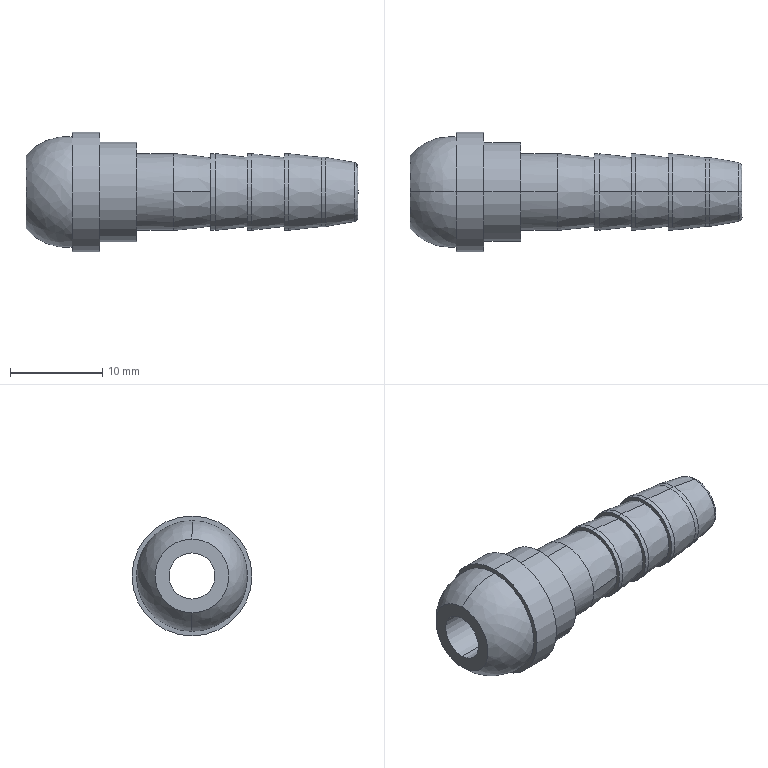Part | STEP file | 20C | 1 solid | 38 faces | box 36 x 13 x 13 mm | volume 1696 mm3 | cylinder 16 | cone 10 | plane 8 | spline 4 | commonest cylinder face diameters 8.3 x4 8.341 x4 5 x2 7.5 x2 10.8 x2 13 x2
STEP:
#1=CARTESIAN_POINT('',(44.153,0.,3.206));
#2=VERTEX_POINT('',#1);
#3=CARTESIAN_POINT('',(44.153,0.,-3.206));
#4=VERTEX_POINT('',#3);
#5=CARTESIAN_POINT('',(44.153,0.,0.));
#6=DIRECTION('',(1.,0.,0.));
#7=DIRECTION('',(0.,0.,1.));
#8=AXIS2_PLACEMENT_3D('',#5,#6,#7);
#9=CIRCLE('',#8,3.206);
#10=EDGE_CURVE('',#2,#4,#9,.T.);
#11=ORIENTED_EDGE('',*,*,#10,.T.);
#12=CARTESIAN_POINT('',(44.566,0.,-2.713));
#13=VERTEX_POINT('',#12);
#14=CARTESIAN_POINT('',(44.066,0.,-2.713));
#15=DIRECTION('',(0.,-1.,0.));
#16=DIRECTION('',(0.,0.,-1.));
#17=AXIS2_PLACEMENT_3D('',#14,#15,#16);
#18=CIRCLE('',#17,0.5);
#19=EDGE_CURVE('',#4,#13,#18,.T.);
#20=ORIENTED_EDGE('',*,*,#19,.T.);
#21=CARTESIAN_POINT('',(44.566,0.,2.713));
#22=VERTEX_POINT('',#21);
#23=CARTESIAN_POINT('',(44.566,0.,-2.713));
#24=CARTESIAN_POINT('',(44.566,-5.427,-2.713));
#25=CARTESIAN_POINT('',(44.566,-5.427,2.713));
#26=CARTESIAN_POINT('',(44.566,0.,2.713));
#27=(BOUNDED_CURVE()B_SPLINE_CURVE(3,(#23,#24,#25,#26),.UNSPECIFIED.,.F.,.F.)B_SPLINE_CURVE_WITH_KNOTS((4,4),(0.,1.),.UNSPECIFIED.)CURVE()GEOMETRIC_REPRESENTATION_ITEM()RATIONAL_B_SPLINE_CURVE((1.,0.3333,0.3333,1.))REPRESENTATION_ITEM(''));
#28=EDGE_CURVE('',#13,#22,#27,.T.);
#29=ORIENTED_EDGE('',*,*,#28,.T.);
#30=CARTESIAN_POINT('',(44.066,0.,2.713));
#31=DIRECTION('',(0.,1.,0.));
#32=DIRECTION('',(0.,0.,1.));
#33=AXIS2_PLACEMENT_3D('',#30,#31,#32);
#34=CIRCLE('',#33,0.5);
#35=EDGE_CURVE('',#2,#22,#34,.T.);
#36=ORIENTED_EDGE('',*,*,#35,.F.);
#37=EDGE_LOOP('',(#11,#20,#29,#36));
#38=FACE_OUTER_BOUND('',#37,.T.);
#39=CARTESIAN_POINT('',(44.153,0.,-3.206));
#40=CARTESIAN_POINT('',(44.153,-6.411,-3.206));
#41=CARTESIAN_POINT('',(44.153,-6.411,3.206));
#42=CARTESIAN_POINT('',(44.153,0.,3.206));
#43=CARTESIAN_POINT('',(44.403,0.,-3.162));
#44=CARTESIAN_POINT('',(44.403,-6.323,-3.162));
#45=CARTESIAN_POINT('',(44.403,-6.323,3.162));
#46=CARTESIAN_POINT('',(44.403,0.,3.162));
#47=CARTESIAN_POINT('',(44.566,0.,-2.967));
#48=CARTESIAN_POINT('',(44.566,-5.934,-2.967));
#49=CARTESIAN_POINT('',(44.566,-5.934,2.967));
#50=CARTESIAN_POINT('',(44.566,0.,2.967));
#51=CARTESIAN_POINT('',(44.566,0.,-2.713));
#52=CARTESIAN_POINT('',(44.566,-5.427,-2.713));
#53=CARTESIAN_POINT('',(44.566,-5.427,2.713));
#54=CARTESIAN_POINT('',(44.566,0.,2.713));
#55=(BOUNDED_SURFACE()B_SPLINE_SURFACE(3,3,((#39,#40,#41,#42),(#43,#44,#45,#46),(#47,#48,#49,#50),(#51,#52,#53,#54)),.UNSPECIFIED.,.F.,.F.,.F.)B_SPLINE_SURFACE_WITH_KNOTS((4,4),(4,4),(0.,1.),(0.,1.),.UNSPECIFIED.)GEOMETRIC_REPRESENTATION_ITEM()RATIONAL_B_SPLINE_SURFACE(((1.,0.3333,0.3333,1.),(0.844,0.2813,0.2813,0.844),(0.844,0.2813,0.2813,0.844),(1.,0.3333,0.3333,1.)))REPRESENTATION_ITEM('')SURFACE());
#56=ADVANCED_FACE('',(#38),#55,.T.);
#57=CARTESIAN_POINT('',(8.566,0.,4.));
#58=VERTEX_POINT('',#57);
#59=CARTESIAN_POINT('',(8.566,0.,-4.));
#60=VERTEX_POINT('',#59);
#61=CARTESIAN_POINT('',(8.566,0.,0.));
#62=DIRECTION('',(1.,0.,0.));
#63=DIRECTION('',(0.,0.,1.));
#64=AXIS2_PLACEMENT_3D('',#61,#62,#63);
#65=CIRCLE('',#64,4.);
#66=EDGE_CURVE('',#58,#60,#65,.T.);
#67=ORIENTED_EDGE('',*,*,#66,.T.);
#68=CARTESIAN_POINT('',(13.566,0.,-6.));
#69=VERTEX_POINT('',#68);
#70=CARTESIAN_POINT('',(13.057,0.,-0.0216));
#71=DIRECTION('',(0.,-1.,0.));
#72=DIRECTION('',(0.,0.,-1.));
#73=AXIS2_PLACEMENT_3D('',#70,#71,#72);
#74=CIRCLE('',#73,6.);
#75=EDGE_CURVE('',#60,#69,#74,.T.);
#76=ORIENTED_EDGE('',*,*,#75,.T.);
#77=CARTESIAN_POINT('',(13.566,0.,6.));
#78=VERTEX_POINT('',#77);
#79=CARTESIAN_POINT('',(13.566,0.,0.));
#80=DIRECTION('',(-1.,0.,0.));
#81=DIRECTION('',(0.,0.,1.));
#82=AXIS2_PLACEMENT_3D('',#79,#80,#81);
#83=CIRCLE('',#82,6.);
#84=EDGE_CURVE('',#69,#78,#83,.T.);
#85=ORIENTED_EDGE('',*,*,#84,.T.);
#86=CARTESIAN_POINT('',(13.057,0.,0.0216));
#87=DIRECTION('',(0.,1.,0.));
#88=DIRECTION('',(0.,0.,1.));
#89=AXIS2_PLACEMENT_3D('',#86,#87,#88);
#90=CIRCLE('',#89,6.);
#91=EDGE_CURVE('',#58,#78,#90,.T.);
#92=ORIENTED_EDGE('',*,*,#91,.F.);
#93=EDGE_LOOP('',(#67,#76,#85,#92));
#94=FACE_OUTER_BOUND('',#93,.T.);
#95=CARTESIAN_POINT('',(8.566,0.,-4.));
#96=CARTESIAN_POINT('',(8.566,-8.,-4.));
#97=CARTESIAN_POINT('',(8.566,-8.,4.));
#98=CARTESIAN_POINT('',(8.566,0.,4.));
#99=CARTESIAN_POINT('',(9.847,0.,-5.446));
#100=CARTESIAN_POINT('',(9.847,-10.892,-5.446));
#101=CARTESIAN_POINT('',(9.847,-10.892,5.446));
#102=CARTESIAN_POINT('',(9.847,0.,5.446));
#103=CARTESIAN_POINT('',(11.641,0.,-6.164));
#104=CARTESIAN_POINT('',(11.641,-12.328,-6.164));
#105=CARTESIAN_POINT('',(11.641,-12.328,6.164));
#106=CARTESIAN_POINT('',(11.641,0.,6.164));
#107=CARTESIAN_POINT('',(13.566,0.,-6.));
#108=CARTESIAN_POINT('',(13.566,-12.,-6.));
#109=CARTESIAN_POINT('',(13.566,-12.,6.));
#110=CARTESIAN_POINT('',(13.566,0.,6.));
#111=(BOUNDED_SURFACE()B_SPLINE_SURFACE(3,3,((#95,#96,#97,#98),(#99,#100,#101,#102),(#103,#104,#105,#106),(#107,#108,#109,#110)),.UNSPECIFIED.,.F.,.F.,.T.)B_SPLINE_SURFACE_WITH_KNOTS((4,4),(4,4),(0.,1.),(0.,1.),.UNSPECIFIED.)GEOMETRIC_REPRESENTATION_ITEM()RATIONAL_B_SPLINE_SURFACE(((1.,0.3333,0.3333,1.),(0.9291,0.3097,0.3097,0.9291),(0.9291,0.3097,0.3097,0.9291),(1.,0.3333,0.3333,1.)))REPRESENTATION_ITEM('')SURFACE());
#112=ADVANCED_FACE('',(#94),#111,.T.);
#113=CARTESIAN_POINT('',(44.566,0.,-2.5));
#114=VERTEX_POINT('',#113);
#115=CARTESIAN_POINT('',(44.566,0.,2.5));
#116=VERTEX_POINT('',#115);
#117=CARTESIAN_POINT('',(44.566,0.,0.));
#118=DIRECTION('',(-1.,0.,0.));
#119=DIRECTION('',(0.,0.,1.));
#120=AXIS2_PLACEMENT_3D('',#117,#118,#119);
#121=CIRCLE('',#120,2.5);
#122=EDGE_CURVE('',#114,#116,#121,.T.);
#123=ORIENTED_EDGE('',*,*,#122,.F.);
#124=CARTESIAN_POINT('',(8.566,0.,-2.5));
#125=VERTEX_POINT('',#124);
#126=CARTESIAN_POINT('',(-40.973,0.,-2.5));
#127=DIRECTION('',(-1.,0.,0.));
#128=VECTOR('',#127,1000.);
#129=LINE('',#126,#128);
#130=EDGE_CURVE('',#114,#125,#129,.T.);
#131=ORIENTED_EDGE('',*,*,#130,.T.);
#132=CARTESIAN_POINT('',(8.566,0.,2.5));
#133=VERTEX_POINT('',#132);
#134=CARTESIAN_POINT('',(8.566,0.,0.));
#135=DIRECTION('',(1.,0.,0.));
#136=DIRECTION('',(0.,0.,1.));
#137=AXIS2_PLACEMENT_3D('',#134,#135,#136);
#138=CIRCLE('',#137,2.5);
#139=EDGE_CURVE('',#133,#125,#138,.T.);
#140=ORIENTED_EDGE('',*,*,#139,.F.);
#141=CARTESIAN_POINT('',(-40.973,0.,2.5));
#142=DIRECTION('',(-1.,0.,0.));
#143=VECTOR('',#142,1000.);
#144=LINE('',#141,#143);
#145=EDGE_CURVE('',#116,#133,#144,.T.);
#146=ORIENTED_EDGE('',*,*,#145,.F.);
#147=EDGE_LOOP('',(#123,#131,#140,#146));
#148=FACE_OUTER_BOUND('',#147,.T.);
#149=CARTESIAN_POINT('',(-40.973,0.,0.));
#150=DIRECTION('',(-1.,0.,0.));
#151=DIRECTION('',(0.,0.,1.));
#152=AXIS2_PLACEMENT_3D('',#149,#150,#151);
#153=CYLINDRICAL_SURFACE('',#152,2.5);
#154=ADVANCED_FACE('',(#148),#153,.F.);
#155=CARTESIAN_POINT('',(44.153,0.,0.));
#156=DIRECTION('',(1.,0.,0.));
#157=DIRECTION('',(0.,0.,1.));
#158=AXIS2_PLACEMENT_3D('',#155,#156,#157);
#159=CIRCLE('',#158,3.206);
#160=EDGE_CURVE('',#4,#2,#159,.T.);
#161=ORIENTED_EDGE('',*,*,#160,.F.);
#162=CARTESIAN_POINT('',(41.066,0.,-3.75));
#163=VERTEX_POINT('',#162);
#164=CARTESIAN_POINT('',(41.066,0.,-3.75));
#165=DIRECTION('',(-0.9848,0.,-0.1736));
#166=VECTOR('',#165,1000.);
#167=LINE('',#164,#166);
#168=EDGE_CURVE('',#4,#163,#167,.T.);
#169=ORIENTED_EDGE('',*,*,#168,.T.);
#170=CARTESIAN_POINT('',(41.066,0.,3.75));
#171=VERTEX_POINT('',#170);
#172=CARTESIAN_POINT('',(41.066,0.,0.));
#173=DIRECTION('',(1.,0.,0.));
#174=DIRECTION('',(0.,0.,1.));
#175=AXIS2_PLACEMENT_3D('',#172,#173,#174);
#176=CIRCLE('',#175,3.75);
#177=EDGE_CURVE('',#163,#171,#176,.T.);
#178=ORIENTED_EDGE('',*,*,#177,.T.);
#179=CARTESIAN_POINT('',(41.066,0.,3.75));
#180=DIRECTION('',(-0.9848,0.,0.1736));
#181=VECTOR('',#180,1000.);
#182=LINE('',#179,#181);
#183=EDGE_CURVE('',#2,#171,#182,.T.);
#184=ORIENTED_EDGE('',*,*,#183,.F.);
#185=EDGE_LOOP('',(#161,#169,#178,#184));
#186=FACE_OUTER_BOUND('',#185,.T.);
#187=CARTESIAN_POINT('',(41.066,0.,0.));
#188=DIRECTION('',(-1.,0.,0.));
#189=DIRECTION('',(0.,0.,1.));
#190=AXIS2_PLACEMENT_3D('',#187,#188,#189);
#191=CONICAL_SURFACE('',#190,3.75,0.1745);
#192=ADVANCED_FACE('',(#186),#191,.T.);
#193=ORIENTED_EDGE('',*,*,#177,.F.);
#194=CARTESIAN_POINT('',(40.566,0.,-3.75));
#195=VERTEX_POINT('',#194);
#196=CARTESIAN_POINT('',(-40.973,0.,-3.75));
#197=DIRECTION('',(-1.,0.,0.));
#198=VECTOR('',#197,1000.);
#199=LINE('',#196,#198);
#200=EDGE_CURVE('',#163,#195,#199,.T.);
#201=ORIENTED_EDGE('',*,*,#200,.T.);
#202=CARTESIAN_POINT('',(40.566,0.,3.75));
#203=VERTEX_POINT('',#202);
#204=CARTESIAN_POINT('',(40.566,0.,0.));
#205=DIRECTION('',(1.,0.,0.));
#206=DIRECTION('',(0.,0.,1.));
#207=AXIS2_PLACEMENT_3D('',#204,#205,#206);
#208=CIRCLE('',#207,3.75);
#209=EDGE_CURVE('',#195,#203,#208,.T.);
#210=ORIENTED_EDGE('',*,*,#209,.T.);
#211=CARTESIAN_POINT('',(-40.973,0.,3.75));
#212=DIRECTION('',(-1.,0.,0.));
#213=VECTOR('',#212,1000.);
#214=LINE('',#211,#213);
#215=EDGE_CURVE('',#171,#203,#214,.T.);
#216=ORIENTED_EDGE('',*,*,#215,.F.);
#217=EDGE_LOOP('',(#193,#201,#210,#216));
#218=FACE_OUTER_BOUND('',#217,.T.);
#219=CARTESIAN_POINT('',(-40.973,0.,0.));
#220=DIRECTION('',(-1.,0.,0.));
#221=DIRECTION('',(0.,0.,1.));
#222=AXIS2_PLACEMENT_3D('',#219,#220,#221);
#223=CYLINDRICAL_SURFACE('',#222,3.75);
#224=ADVANCED_FACE('',(#218),#223,.T.);
#225=CARTESIAN_POINT('',(16.566,0.,6.5));
#226=VERTEX_POINT('',#225);
#227=CARTESIAN_POINT('',(16.566,0.,-6.5));
#228=VERTEX_POINT('',#227);
#229=CARTESIAN_POINT('',(16.566,0.,0.));
#230=DIRECTION('',(-1.,0.,0.));
#231=DIRECTION('',(0.,0.,1.));
#232=AXIS2_PLACEMENT_3D('',#229,#230,#231);
#233=CIRCLE('',#232,6.5);
#234=EDGE_CURVE('',#226,#228,#233,.T.);
#235=ORIENTED_EDGE('',*,*,#234,.T.);
#236=CARTESIAN_POINT('',(13.566,0.,-6.5));
#237=VERTEX_POINT('',#236);
#238=CARTESIAN_POINT('',(-40.973,0.,-6.5));
#239=DIRECTION('',(-1.,0.,0.));
#240=VECTOR('',#239,1000.);
#241=LINE('',#238,#240);
#242=EDGE_CURVE('',#228,#237,#241,.T.);
#243=ORIENTED_EDGE('',*,*,#242,.T.);
#244=CARTESIAN_POINT('',(13.566,0.,6.5));
#245=VERTEX_POINT('',#244);
#246=CARTESIAN_POINT('',(13.566,0.,0.));
#247=DIRECTION('',(1.,0.,0.));
#248=DIRECTION('',(0.,0.,1.));
#249=AXIS2_PLACEMENT_3D('',#246,#247,#248);
#250=CIRCLE('',#249,6.5);
#251=EDGE_CURVE('',#237,#245,#250,.T.);
#252=ORIENTED_EDGE('',*,*,#251,.T.);
#253=CARTESIAN_POINT('',(-40.973,0.,6.5));
#254=DIRECTION('',(-1.,0.,0.));
#255=VECTOR('',#254,1000.);
#256=LINE('',#253,#255);
#257=EDGE_CURVE('',#226,#245,#256,.T.);
#258=ORIENTED_EDGE('',*,*,#257,.F.);
#259=EDGE_LOOP('',(#235,#243,#252,#258));
#260=FACE_OUTER_BOUND('',#259,.T.);
#261=CARTESIAN_POINT('',(-40.973,0.,0.));
#262=DIRECTION('',(-1.,0.,0.));
#263=DIRECTION('',(0.,0.,1.));
#264=AXIS2_PLACEMENT_3D('',#261,#262,#263);
#265=CYLINDRICAL_SURFACE('',#264,6.5);
#266=ADVANCED_FACE('',(#260),#265,.T.);
#267=ORIENTED_EDGE('',*,*,#209,.F.);
#268=CARTESIAN_POINT('',(37.066,0.,-4.15));
#269=VERTEX_POINT('',#268);
#270=CARTESIAN_POINT('',(37.066,0.,-4.15));
#271=DIRECTION('',(-0.9935,0.,-0.1135));
#272=VECTOR('',#271,1000.);
#273=LINE('',#270,#272);
#274=EDGE_CURVE('',#195,#269,#273,.T.);
#275=ORIENTED_EDGE('',*,*,#274,.T.);
#276=CARTESIAN_POINT('',(37.066,0.,4.15));
#277=VERTEX_POINT('',#276);
#278=CARTESIAN_POINT('',(37.066,0.,0.));
#279=DIRECTION('',(1.,0.,0.));
#280=DIRECTION('',(0.,0.,1.));
#281=AXIS2_PLACEMENT_3D('',#278,#279,#280);
#282=CIRCLE('',#281,4.15);
#283=EDGE_CURVE('',#269,#277,#282,.T.);
#284=ORIENTED_EDGE('',*,*,#283,.T.);
#285=CARTESIAN_POINT('',(37.066,0.,4.15));
#286=DIRECTION('',(-0.9935,0.,0.1135));
#287=VECTOR('',#286,1000.);
#288=LINE('',#285,#287);
#289=EDGE_CURVE('',#203,#277,#288,.T.);
#290=ORIENTED_EDGE('',*,*,#289,.F.);
#291=EDGE_LOOP('',(#267,#275,#284,#290));
#292=FACE_OUTER_BOUND('',#291,.T.);
#293=CARTESIAN_POINT('',(37.066,0.,0.));
#294=DIRECTION('',(-1.,0.,0.));
#295=DIRECTION('',(0.,0.,1.));
#296=AXIS2_PLACEMENT_3D('',#293,#294,#295);
#297=CONICAL_SURFACE('',#296,4.15,0.1138);
#298=ADVANCED_FACE('',(#292),#297,.T.);
#299=ORIENTED_EDGE('',*,*,#283,.F.);
#300=CARTESIAN_POINT('',(36.566,0.,-4.15));
#301=VERTEX_POINT('',#300);
#302=CARTESIAN_POINT('',(-40.973,0.,-4.15));
#303=DIRECTION('',(-1.,0.,0.));
#304=VECTOR('',#303,1000.);
#305=LINE('',#302,#304);
#306=EDGE_CURVE('',#269,#301,#305,.T.);
#307=ORIENTED_EDGE('',*,*,#306,.T.);
#308=CARTESIAN_POINT('',(36.566,0.,4.15));
#309=VERTEX_POINT('',#308);
#310=CARTESIAN_POINT('',(36.566,0.,0.));
#311=DIRECTION('',(1.,0.,0.));
#312=DIRECTION('',(0.,0.,1.));
#313=AXIS2_PLACEMENT_3D('',#310,#311,#312);
#314=CIRCLE('',#313,4.15);
#315=EDGE_CURVE('',#301,#309,#314,.T.);
#316=ORIENTED_EDGE('',*,*,#315,.T.);
#317=CARTESIAN_POINT('',(-40.973,0.,4.15));
#318=DIRECTION('',(-1.,0.,0.));
#319=VECTOR('',#318,1000.);
#320=LINE('',#317,#319);
#321=EDGE_CURVE('',#277,#309,#320,.T.);
#322=ORIENTED_EDGE('',*,*,#321,.F.);
#323=EDGE_LOOP('',(#299,#307,#316,#322));
#324=FACE_OUTER_BOUND('',#323,.T.);
#325=CARTESIAN_POINT('',(-40.973,0.,0.));
#326=DIRECTION('',(-1.,0.,0.));
#327=DIRECTION('',(0.,0.,1.));
#328=AXIS2_PLACEMENT_3D('',#325,#326,#327);
#329=CYLINDRICAL_SURFACE('',#328,4.15);
#330=ADVANCED_FACE('',(#324),#329,.T.);
#331=CARTESIAN_POINT('',(20.566,0.,5.4));
#332=VERTEX_POINT('',#331);
#333=CARTESIAN_POINT('',(20.566,0.,-5.4));
#334=VERTEX_POINT('',#333);
#335=CARTESIAN_POINT('',(20.566,0.,0.));
#336=DIRECTION('',(-1.,0.,0.));
#337=DIRECTION('',(0.,0.,1.));
#338=AXIS2_PLACEMENT_3D('',#335,#336,#337);
#339=CIRCLE('',#338,5.4);
#340=EDGE_CURVE('',#332,#334,#339,.T.);
#341=ORIENTED_EDGE('',*,*,#340,.T.);
#342=CARTESIAN_POINT('',(16.566,0.,-5.4));
#343=VERTEX_POINT('',#342);
#344=CARTESIAN_POINT('',(-40.973,0.,-5.4));
#345=DIRECTION('',(-1.,0.,0.));
#346=VECTOR('',#345,1000.);
#347=LINE('',#344,#346);
#348=EDGE_CURVE('',#334,#343,#347,.T.);
#349=ORIENTED_EDGE('',*,*,#348,.T.);
#350=CARTESIAN_POINT('',(16.566,0.,5.4));
#351=VERTEX_POINT('',#350);
#352=CARTESIAN_POINT('',(16.566,0.,0.));
#353=DIRECTION('',(1.,0.,0.));
#354=DIRECTION('',(0.,0.,1.));
#355=AXIS2_PLACEMENT_3D('',#352,#353,#354);
#356=CIRCLE('',#355,5.4);
#357=EDGE_CURVE('',#343,#351,#356,.T.);
#358=ORIENTED_EDGE('',*,*,#357,.T.);
#359=CARTESIAN_POINT('',(-40.973,0.,5.4));
#360=DIRECTION('',(-1.,0.,0.));
#361=VECTOR('',#360,1000.);
#362=LINE('',#359,#361);
#363=EDGE_CURVE('',#332,#351,#362,.T.);
#364=ORIENTED_EDGE('',*,*,#363,.F.);
#365=EDGE_LOOP('',(#341,#349,#358,#364));
#366=FACE_OUTER_BOUND('',#365,.T.);
#367=CARTESIAN_POINT('',(-40.973,0.,0.));
#368=DIRECTION('',(-1.,0.,0.));
#369=DIRECTION('',(0.,0.,1.));
#370=AXIS2_PLACEMENT_3D('',#367,#368,#369);
#371=CYLINDRICAL_SURFACE('',#370,5.4);
#372=ADVANCED_FACE('',(#366),#371,.T.);
#373=CARTESIAN_POINT('',(36.566,0.,3.73));
#374=VERTEX_POINT('',#373);
#375=CARTESIAN_POINT('',(36.566,0.,-3.73));
#376=VERTEX_POINT('',#375);
#377=CARTESIAN_POINT('',(36.566,0.,0.));
#378=DIRECTION('',(-1.,0.,0.));
#379=DIRECTION('',(0.,0.,1.));
#380=AXIS2_PLACEMENT_3D('',#377,#378,#379);
#381=CIRCLE('',#380,3.73);
#382=EDGE_CURVE('',#374,#376,#381,.T.);
#383=ORIENTED_EDGE('',*,*,#382,.T.);
#384=CARTESIAN_POINT('',(33.066,0.,-4.15));
#385=VERTEX_POINT('',#384);
#386=CARTESIAN_POINT('',(33.066,0.,-4.15));
#387=DIRECTION('',(-0.9929,0.,-0.1192));
#388=VECTOR('',#387,1000.);
#389=LINE('',#386,#388);
#390=EDGE_CURVE('',#376,#385,#389,.T.);
#391=ORIENTED_EDGE('',*,*,#390,.T.);
#392=CARTESIAN_POINT('',(33.066,0.,4.15));
#393=VERTEX_POINT('',#392);
#394=CARTESIAN_POINT('',(33.066,0.,0.));
#395=DIRECTION('',(1.,0.,0.));
#396=DIRECTION('',(0.,0.,1.));
#397=AXIS2_PLACEMENT_3D('',#394,#395,#396);
#398=CIRCLE('',#397,4.15);
#399=EDGE_CURVE('',#385,#393,#398,.T.);
#400=ORIENTED_EDGE('',*,*,#399,.T.);
#401=CARTESIAN_POINT('',(33.066,0.,4.15));
#402=DIRECTION('',(-0.9929,0.,0.1192));
#403=VECTOR('',#402,1000.);
#404=LINE('',#401,#403);
#405=EDGE_CURVE('',#374,#393,#404,.T.);
#406=ORIENTED_EDGE('',*,*,#405,.F.);
#407=EDGE_LOOP('',(#383,#391,#400,#406));
#408=FACE_OUTER_BOUND('',#407,.T.);
#409=CARTESIAN_POINT('',(33.066,0.,0.));
#410=DIRECTION('',(-1.,0.,0.));
#411=DIRECTION('',(0.,0.,1.));
#412=AXIS2_PLACEMENT_3D('',#409,#410,#411);
#413=CONICAL_SURFACE('',#412,4.15,0.1195);
#414=ADVANCED_FACE('',(#408),#413,.T.);
#415=CARTESIAN_POINT('',(24.566,4.17,0.));
#416=VERTEX_POINT('',#415);
#417=CARTESIAN_POINT('',(24.566,0.,-4.17));
#418=VERTEX_POINT('',#417);
#419=CARTESIAN_POINT('',(24.566,0.,0.));
#420=DIRECTION('',(-1.,0.,0.));
#421=DIRECTION('',(0.,0.,1.));
#422=AXIS2_PLACEMENT_3D('',#419,#420,#421);
#423=CIRCLE('',#422,4.17);
#424=EDGE_CURVE('',#416,#418,#423,.T.);
#425=ORIENTED_EDGE('',*,*,#424,.T.);
#426=CARTESIAN_POINT('',(20.566,0.,-4.17));
#427=VERTEX_POINT('',#426);
#428=CARTESIAN_POINT('',(-40.973,0.,-4.17));
#429=DIRECTION('',(-1.,0.,0.));
#430=VECTOR('',#429,1000.);
#431=LINE('',#428,#430);
#432=EDGE_CURVE('',#418,#427,#431,.T.);
#433=ORIENTED_EDGE('',*,*,#432,.T.);
#434=CARTESIAN_POINT('',(20.566,0.,4.17));
#435=VERTEX_POINT('',#434);
#436=CARTESIAN_POINT('',(20.566,0.,0.));
#437=DIRECTION('',(1.,0.,0.));
#438=DIRECTION('',(0.,0.,1.));
#439=AXIS2_PLACEMENT_3D('',#436,#437,#438);
#440=CIRCLE('',#439,4.17);
#441=EDGE_CURVE('',#427,#435,#440,.T.);
#442=ORIENTED_EDGE('',*,*,#441,.T.);
#443=CARTESIAN_POINT('',(24.566,0.,4.17));
#444=VERTEX_POINT('',#443);
#445=CARTESIAN_POINT('',(-40.973,0.,4.17));
#446=DIRECTION('',(-1.,0.,0.));
#447=VECTOR('',#446,1000.);
#448=LINE('',#445,#447);
#449=EDGE_CURVE('',#444,#435,#448,.T.);
#450=ORIENTED_EDGE('',*,*,#449,.F.);
#451=CARTESIAN_POINT('',(24.566,0.,0.));
#452=DIRECTION('',(-1.,0.,0.));
#453=DIRECTION('',(0.,0.,1.));
#454=AXIS2_PLACEMENT_3D('',#451,#452,#453);
#455=CIRCLE('',#454,4.17);
#456=EDGE_CURVE('',#444,#416,#455,.T.);
#457=ORIENTED_EDGE('',*,*,#456,.T.);
#458=EDGE_LOOP('',(#425,#433,#442,#450,#457));
#459=FACE_OUTER_BOUND('',#458,.T.);
#460=CARTESIAN_POINT('',(-40.973,0.,0.));
#461=DIRECTION('',(-1.,0.,0.));
#462=DIRECTION('',(0.,0.,1.));
#463=AXIS2_PLACEMENT_3D('',#460,#461,#462);
#464=CYLINDRICAL_SURFACE('',#463,4.17);
#465=ADVANCED_FACE('',(#459),#464,.T.);
#466=ORIENTED_EDGE('',*,*,#399,.F.);
#467=CARTESIAN_POINT('',(32.566,0.,-4.15));
#468=VERTEX_POINT('',#467);
#469=CARTESIAN_POINT('',(-40.973,0.,-4.15));
#470=DIRECTION('',(-1.,0.,0.));
#471=VECTOR('',#470,1000.);
#472=LINE('',#469,#471);
#473=EDGE_CURVE('',#385,#468,#472,.T.);
#474=ORIENTED_EDGE('',*,*,#473,.T.);
#475=CARTESIAN_POINT('',(32.566,0.,4.15));
#476=VERTEX_POINT('',#475);
#477=CARTESIAN_POINT('',(32.566,0.,0.));
#478=DIRECTION('',(1.,0.,0.));
#479=DIRECTION('',(0.,0.,1.));
#480=AXIS2_PLACEMENT_3D('',#477,#478,#479);
#481=CIRCLE('',#480,4.15);
#482=EDGE_CURVE('',#468,#476,#481,.T.);
#483=ORIENTED_EDGE('',*,*,#482,.T.);
#484=CARTESIAN_POINT('',(-40.973,0.,4.15));
#485=DIRECTION('',(-1.,0.,0.));
#486=VECTOR('',#485,1000.);
#487=LINE('',#484,#486);
#488=EDGE_CURVE('',#393,#476,#487,.T.);
#489=ORIENTED_EDGE('',*,*,#488,.F.);
#490=EDGE_LOOP('',(#466,#474,#483,#489));
#491=FACE_OUTER_BOUND('',#490,.T.);
#492=CARTESIAN_POINT('',(-40.973,0.,0.));
#493=DIRECTION('',(-1.,0.,0.));
#494=DIRECTION('',(0.,0.,1.));
#495=AXIS2_PLACEMENT_3D('',#492,#493,#494);
#496=CYLINDRICAL_SURFACE('',#495,4.15);
#497=ADVANCED_FACE('',(#491),#496,.T.);
#498=CARTESIAN_POINT('',(28.566,-3.734,0.));
#499=VERTEX_POINT('',#498);
#500=CARTESIAN_POINT('',(28.566,3.734,0.));
#501=VERTEX_POINT('',#500);
#502=CARTESIAN_POINT('',(28.566,0.,0.));
#503=DIRECTION('',(-1.,0.,0.));
#504=DIRECTION('',(0.,-1.,0.));
#505=AXIS2_PLACEMENT_3D('',#502,#503,#504);
#506=CIRCLE('',#505,3.734);
#507=EDGE_CURVE('',#499,#501,#506,.T.);
#508=ORIENTED_EDGE('',*,*,#507,.T.);
#509=CARTESIAN_POINT('',(24.566,4.17,0.));
#510=DIRECTION('',(-0.9941,0.1084,0.));
#511=VECTOR('',#510,1000.);
#512=LINE('',#509,#511);
#513=EDGE_CURVE('',#501,#416,#512,.T.);
#514=ORIENTED_EDGE('',*,*,#513,.T.);
#515=ORIENTED_EDGE('',*,*,#456,.F.);
#516=CARTESIAN_POINT('',(24.566,-4.17,0.));
#517=VERTEX_POINT('',#516);
#518=CARTESIAN_POINT('',(24.566,0.,0.));
#519=DIRECTION('',(-1.,0.,0.));
#520=DIRECTION('',(0.,0.,1.));
#521=AXIS2_PLACEMENT_3D('',#518,#519,#520);
#522=CIRCLE('',#521,4.17);
#523=EDGE_CURVE('',#517,#444,#522,.T.);
#524=ORIENTED_EDGE('',*,*,#523,.F.);
#525=CARTESIAN_POINT('',(24.566,-4.17,0.));
#526=DIRECTION('',(-0.9941,-0.1084,0.));
#527=VECTOR('',#526,1000.);
#528=LINE('',#525,#527);
#529=EDGE_CURVE('',#499,#517,#528,.T.);
#530=ORIENTED_EDGE('',*,*,#529,.F.);
#531=EDGE_LOOP('',(#508,#514,#515,#524,#530));
#532=FACE_OUTER_BOUND('',#531,.T.);
#533=CARTESIAN_POINT('',(24.566,0.,0.));
#534=DIRECTION('',(-1.,0.,0.));
#535=DIRECTION('',(0.,-1.,0.));
#536=AXIS2_PLACEMENT_3D('',#533,#534,#535);
#537=CONICAL_SURFACE('',#536,4.17,0.1086);
#538=ADVANCED_FACE('',(#532),#537,.T.);
#539=CARTESIAN_POINT('',(32.566,0.,3.75));
#540=VERTEX_POINT('',#539);
#541=CARTESIAN_POINT('',(32.566,0.,-3.75));
#542=VERTEX_POINT('',#541);
#543=CARTESIAN_POINT('',(32.566,0.,0.));
#544=DIRECTION('',(-1.,0.,0.));
#545=DIRECTION('',(0.,0.,1.));
#546=AXIS2_PLACEMENT_3D('',#543,#544,#545);
#547=CIRCLE('',#546,3.75);
#548=EDGE_CURVE('',#540,#542,#547,.T.);
#549=ORIENTED_EDGE('',*,*,#548,.T.);
#550=CARTESIAN_POINT('',(29.066,0.,-4.17));
#551=VERTEX_POINT('',#550);
#552=CARTESIAN_POINT('',(29.066,0.,-4.17));
#553=DIRECTION('',(-0.9929,0.,-0.1192));
#554=VECTOR('',#553,1000.);
#555=LINE('',#552,#554);
#556=EDGE_CURVE('',#542,#551,#555,.T.);
#557=ORIENTED_EDGE('',*,*,#556,.T.);
#558=CARTESIAN_POINT('',(29.066,0.,4.17));
#559=VERTEX_POINT('',#558);
#560=CARTESIAN_POINT('',(29.066,0.,0.));
#561=DIRECTION('',(1.,0.,0.));
#562=DIRECTION('',(0.,0.,1.));
#563=AXIS2_PLACEMENT_3D('',#560,#561,#562);
#564=CIRCLE('',#563,4.17);
#565=EDGE_CURVE('',#551,#559,#564,.T.);
#566=ORIENTED_EDGE('',*,*,#565,.T.);
#567=CARTESIAN_POINT('',(29.066,0.,4.17));
#568=DIRECTION('',(-0.9929,0.,0.1192));
#569=VECTOR('',#568,1000.);
#570=LINE('',#567,#569);
#571=EDGE_CURVE('',#540,#559,#570,.T.);
#572=ORIENTED_EDGE('',*,*,#571,.F.);
#573=EDGE_LOOP('',(#549,#557,#566,#572));
#574=FACE_OUTER_BOUND('',#573,.T.);
#575=CARTESIAN_POINT('',(29.066,0.,0.));
#576=DIRECTION('',(-1.,0.,0.));
#577=DIRECTION('',(0.,0.,1.));
#578=AXIS2_PLACEMENT_3D('',#575,#576,#577);
#579=CONICAL_SURFACE('',#578,4.17,0.1195);
#580=ADVANCED_FACE('',(#574),#579,.T.);
#581=ORIENTED_EDGE('',*,*,#565,.F.);
#582=CARTESIAN_POINT('',(28.566,0.,-4.17));
#583=VERTEX_POINT('',#582);
#584=CARTESIAN_POINT('',(-40.973,0.,-4.17));
#585=DIRECTION('',(-1.,0.,0.));
#586=VECTOR('',#585,1000.);
#587=LINE('',#584,#586);
#588=EDGE_CURVE('',#551,#583,#587,.T.);
#589=ORIENTED_EDGE('',*,*,#588,.T.);
#590=CARTESIAN_POINT('',(28.566,0.,4.17));
#591=VERTEX_POINT('',#590);
#592=CARTESIAN_POINT('',(28.566,0.,0.));
#593=DIRECTION('',(1.,0.,0.));
#594=DIRECTION('',(0.,0.,1.));
#595=AXIS2_PLACEMENT_3D('',#592,#593,#594);
#596=CIRCLE('',#595,4.17);
#597=EDGE_CURVE('',#583,#591,#596,.T.);
#598=ORIENTED_EDGE('',*,*,#597,.T.);
#599=CARTESIAN_POINT('',(-40.973,0.,4.17));
#600=DIRECTION('',(-1.,0.,0.));
#601=VECTOR('',#600,1000.);
#602=LINE('',#599,#601);
#603=EDGE_CURVE('',#559,#591,#602,.T.);
#604=ORIENTED_EDGE('',*,*,#603,.F.);
#605=EDGE_LOOP('',(#581,#589,#598,#604));
#606=FACE_OUTER_BOUND('',#605,.T.);
#607=CARTESIAN_POINT('',(-40.973,0.,0.));
#608=DIRECTION('',(-1.,0.,0.));
#609=DIRECTION('',(0.,0.,1.));
#610=AXIS2_PLACEMENT_3D('',#607,#608,#609);
#611=CYLINDRICAL_SURFACE('',#610,4.17);
#612=ADVANCED_FACE('',(#606),#611,.T.);
#613=ORIENTED_EDGE('',*,*,#130,.F.);
#614=CARTESIAN_POINT('',(44.566,0.,0.));
#615=DIRECTION('',(-1.,0.,0.));
#616=DIRECTION('',(0.,0.,1.));
#617=AXIS2_PLACEMENT_3D('',#614,#615,#616);
#618=CIRCLE('',#617,2.5);
#619=EDGE_CURVE('',#116,#114,#618,.T.);
#620=ORIENTED_EDGE('',*,*,#619,.F.);
#621=ORIENTED_EDGE('',*,*,#145,.T.);
#622=CARTESIAN_POINT('',(8.566,0.,0.));
#623=DIRECTION('',(1.,0.,0.));
#624=DIRECTION('',(0.,0.,1.));
#625=AXIS2_PLACEMENT_3D('',#622,#623,#624);
#626=CIRCLE('',#625,2.5);
#627=EDGE_CURVE('',#125,#133,#626,.T.);
#628=ORIENTED_EDGE('',*,*,#627,.F.);
#629=EDGE_LOOP('',(#613,#620,#621,#628));
#630=FACE_OUTER_BOUND('',#629,.T.);
#631=CARTESIAN_POINT('',(-40.973,0.,0.));
#632=DIRECTION('',(-1.,0.,0.));
#633=DIRECTION('',(0.,0.,1.));
#634=AXIS2_PLACEMENT_3D('',#631,#632,#633);
#635=CYLINDRICAL_SURFACE('',#634,2.5);
#636=ADVANCED_FACE('',(#630),#635,.F.);
#637=ORIENTED_EDGE('',*,*,#619,.T.);
#638=ORIENTED_EDGE('',*,*,#122,.T.);
#639=EDGE_LOOP('',(#637,#638));
#640=FACE_BOUND('',#639,.T.);
#641=ORIENTED_EDGE('',*,*,#28,.F.);
#642=CARTESIAN_POINT('',(44.566,0.,2.713));
#643=CARTESIAN_POINT('',(44.566,5.427,2.713));
#644=CARTESIAN_POINT('',(44.566,5.427,-2.713));
#645=CARTESIAN_POINT('',(44.566,0.,-2.713));
#646=(BOUNDED_CURVE()B_SPLINE_CURVE(3,(#642,#643,#644,#645),.UNSPECIFIED.,.F.,.F.)B_SPLINE_CURVE_WITH_KNOTS((4,4),(0.,1.),.UNSPECIFIED.)CURVE()GEOMETRIC_REPRESENTATION_ITEM()RATIONAL_B_SPLINE_CURVE((1.,0.3333,0.3333,1.))REPRESENTATION_ITEM(''));
#647=EDGE_CURVE('',#22,#13,#646,.T.);
#648=ORIENTED_EDGE('',*,*,#647,.F.);
#649=EDGE_LOOP('',(#641,#648));
#650=FACE_OUTER_BOUND('',#649,.T.);
#651=CARTESIAN_POINT('',(44.566,0.,-2.5));
#652=DIRECTION('',(-1.,0.,0.));
#653=DIRECTION('',(0.,0.,1.));
#654=AXIS2_PLACEMENT_3D('',#651,#652,#653);
#655=PLANE('',#654);
#656=ADVANCED_FACE('',(#640,#650),#655,.F.);
#657=ORIENTED_EDGE('',*,*,#66,.F.);
#658=CARTESIAN_POINT('',(8.566,0.,0.));
#659=DIRECTION('',(1.,0.,0.));
#660=DIRECTION('',(0.,0.,1.));
#661=AXIS2_PLACEMENT_3D('',#658,#659,#660);
#662=CIRCLE('',#661,4.);
#663=EDGE_CURVE('',#60,#58,#662,.T.);
#664=ORIENTED_EDGE('',*,*,#663,.F.);
#665=EDGE_LOOP('',(#657,#664));
#666=FACE_OUTER_BOUND('',#665,.T.);
#667=ORIENTED_EDGE('',*,*,#139,.T.);
#668=ORIENTED_EDGE('',*,*,#627,.T.);
#669=EDGE_LOOP('',(#667,#668));
#670=FACE_BOUND('',#669,.T.);
#671=CARTESIAN_POINT('',(8.566,0.,-2.5));
#672=DIRECTION('',(1.,0.,0.));
#673=DIRECTION('',(0.,0.,-1.));
#674=AXIS2_PLACEMENT_3D('',#671,#672,#673);
#675=PLANE('',#674);
#676=ADVANCED_FACE('',(#666,#670),#675,.F.);
#677=ORIENTED_EDGE('',*,*,#19,.F.);
#678=ORIENTED_EDGE('',*,*,#160,.T.);
#679=ORIENTED_EDGE('',*,*,#35,.T.);
#680=ORIENTED_EDGE('',*,*,#647,.T.);
#681=EDGE_LOOP('',(#677,#678,#679,#680));
#682=FACE_OUTER_BOUND('',#681,.T.);
#683=CARTESIAN_POINT('',(44.153,0.,3.206));
#684=CARTESIAN_POINT('',(44.153,6.411,3.206));
#685=CARTESIAN_POINT('',(44.153,6.411,-3.206));
#686=CARTESIAN_POINT('',(44.153,0.,-3.206));
#687=CARTESIAN_POINT('',(44.403,0.,3.162));
#688=CARTESIAN_POINT('',(44.403,6.323,3.162));
#689=CARTESIAN_POINT('',(44.403,6.323,-3.162));
#690=CARTESIAN_POINT('',(44.403,0.,-3.162));
#691=CARTESIAN_POINT('',(44.566,0.,2.967));
#692=CARTESIAN_POINT('',(44.566,5.934,2.967));
#693=CARTESIAN_POINT('',(44.566,5.934,-2.967));
#694=CARTESIAN_POINT('',(44.566,0.,-2.967));
#695=CARTESIAN_POINT('',(44.566,0.,2.713));
#696=CARTESIAN_POINT('',(44.566,5.427,2.713));
#697=CARTESIAN_POINT('',(44.566,5.427,-2.713));
#698=CARTESIAN_POINT('',(44.566,0.,-2.713));
#699=(BOUNDED_SURFACE()B_SPLINE_SURFACE(3,3,((#683,#684,#685,#686),(#687,#688,#689,#690),(#691,#692,#693,#694),(#695,#696,#697,#698)),.UNSPECIFIED.,.F.,.F.,.F.)B_SPLINE_SURFACE_WITH_KNOTS((4,4),(4,4),(0.,1.),(0.,1.),.UNSPECIFIED.)GEOMETRIC_REPRESENTATION_ITEM()RATIONAL_B_SPLINE_SURFACE(((1.,0.3333,0.3333,1.),(0.844,0.2813,0.2813,0.844),(0.844,0.2813,0.2813,0.844),(1.,0.3333,0.3333,1.)))REPRESENTATION_ITEM('')SURFACE());
#700=ADVANCED_FACE('',(#682),#699,.T.);
#701=ORIENTED_EDGE('',*,*,#75,.F.);
#702=ORIENTED_EDGE('',*,*,#663,.T.);
#703=ORIENTED_EDGE('',*,*,#91,.T.);
#704=CARTESIAN_POINT('',(13.566,0.,0.));
#705=DIRECTION('',(-1.,0.,0.));
#706=DIRECTION('',(0.,0.,1.));
#707=AXIS2_PLACEMENT_3D('',#704,#705,#706);
#708=CIRCLE('',#707,6.);
#709=EDGE_CURVE('',#78,#69,#708,.T.);
#710=ORIENTED_EDGE('',*,*,#709,.T.);
#711=EDGE_LOOP('',(#701,#702,#703,#710));
#712=FACE_OUTER_BOUND('',#711,.T.);
#713=CARTESIAN_POINT('',(8.566,0.,4.));
#714=CARTESIAN_POINT('',(8.566,8.,4.));
#715=CARTESIAN_POINT('',(8.566,8.,-4.));
#716=CARTESIAN_POINT('',(8.566,0.,-4.));
#717=CARTESIAN_POINT('',(9.847,0.,5.446));
#718=CARTESIAN_POINT('',(9.847,10.892,5.446));
#719=CARTESIAN_POINT('',(9.847,10.892,-5.446));
#720=CARTESIAN_POINT('',(9.847,0.,-5.446));
#721=CARTESIAN_POINT('',(11.641,0.,6.164));
#722=CARTESIAN_POINT('',(11.641,12.328,6.164));
#723=CARTESIAN_POINT('',(11.641,12.328,-6.164));
#724=CARTESIAN_POINT('',(11.641,0.,-6.164));
#725=CARTESIAN_POINT('',(13.566,0.,6.));
#726=CARTESIAN_POINT('',(13.566,12.,6.));
#727=CARTESIAN_POINT('',(13.566,12.,-6.));
#728=CARTESIAN_POINT('',(13.566,0.,-6.));
#729=(BOUNDED_SURFACE()B_SPLINE_SURFACE(3,3,((#713,#714,#715,#716),(#717,#718,#719,#720),(#721,#722,#723,#724),(#725,#726,#727,#728)),.UNSPECIFIED.,.F.,.F.,.F.)B_SPLINE_SURFACE_WITH_KNOTS((4,4),(4,4),(0.,1.),(0.,1.),.UNSPECIFIED.)GEOMETRIC_REPRESENTATION_ITEM()RATIONAL_B_SPLINE_SURFACE(((1.,0.3333,0.3333,1.),(0.9291,0.3097,0.3097,0.9291),(0.9291,0.3097,0.3097,0.9291),(1.,0.3333,0.3333,1.)))REPRESENTATION_ITEM('')SURFACE());
#730=ADVANCED_FACE('',(#712),#729,.T.);
#731=ORIENTED_EDGE('',*,*,#168,.F.);
#732=ORIENTED_EDGE('',*,*,#10,.F.);
#733=ORIENTED_EDGE('',*,*,#183,.T.);
#734=CARTESIAN_POINT('',(41.066,0.,0.));
#735=DIRECTION('',(1.,0.,0.));
#736=DIRECTION('',(0.,0.,1.));
#737=AXIS2_PLACEMENT_3D('',#734,#735,#736);
#738=CIRCLE('',#737,3.75);
#739=EDGE_CURVE('',#171,#163,#738,.T.);
#740=ORIENTED_EDGE('',*,*,#739,.T.);
#741=EDGE_LOOP('',(#731,#732,#733,#740));
#742=FACE_OUTER_BOUND('',#741,.T.);
#743=CARTESIAN_POINT('',(41.066,0.,0.));
#744=DIRECTION('',(-1.,0.,0.));
#745=DIRECTION('',(0.,0.,1.));
#746=AXIS2_PLACEMENT_3D('',#743,#744,#745);
#747=CONICAL_SURFACE('',#746,3.75,0.1745);
#748=ADVANCED_FACE('',(#742),#747,.T.);
#749=CARTESIAN_POINT('',(13.566,0.,0.));
#750=DIRECTION('',(1.,0.,0.));
#751=DIRECTION('',(0.,0.,1.));
#752=AXIS2_PLACEMENT_3D('',#749,#750,#751);
#753=CIRCLE('',#752,6.5);
#754=EDGE_CURVE('',#245,#237,#753,.T.);
#755=ORIENTED_EDGE('',*,*,#754,.F.);
#756=ORIENTED_EDGE('',*,*,#251,.F.);
#757=EDGE_LOOP('',(#755,#756));
#758=FACE_OUTER_BOUND('',#757,.T.);
#759=ORIENTED_EDGE('',*,*,#709,.F.);
#760=ORIENTED_EDGE('',*,*,#84,.F.);
#761=EDGE_LOOP('',(#759,#760));
#762=FACE_BOUND('',#761,.T.);
#763=CARTESIAN_POINT('',(13.566,0.,-6.5));
#764=DIRECTION('',(1.,0.,0.));
#765=DIRECTION('',(0.,0.,-1.));
#766=AXIS2_PLACEMENT_3D('',#763,#764,#765);
#767=PLANE('',#766);
#768=ADVANCED_FACE('',(#758,#762),#767,.F.);
#769=ORIENTED_EDGE('',*,*,#200,.F.);
#770=ORIENTED_EDGE('',*,*,#739,.F.);
#771=ORIENTED_EDGE('',*,*,#215,.T.);
#772=CARTESIAN_POINT('',(40.566,0.,0.));
#773=DIRECTION('',(1.,0.,0.));
#774=DIRECTION('',(0.,0.,1.));
#775=AXIS2_PLACEMENT_3D('',#772,#773,#774);
#776=CIRCLE('',#775,3.75);
#777=EDGE_CURVE('',#203,#195,#776,.T.);
#778=ORIENTED_EDGE('',*,*,#777,.T.);
#779=EDGE_LOOP('',(#769,#770,#771,#778));
#780=FACE_OUTER_BOUND('',#779,.T.);
#781=CARTESIAN_POINT('',(-40.973,0.,0.));
#782=DIRECTION('',(-1.,0.,0.));
#783=DIRECTION('',(0.,0.,1.));
#784=AXIS2_PLACEMENT_3D('',#781,#782,#783);
#785=CYLINDRICAL_SURFACE('',#784,3.75);
#786=ADVANCED_FACE('',(#780),#785,.T.);
#787=ORIENTED_EDGE('',*,*,#242,.F.);
#788=CARTESIAN_POINT('',(16.566,0.,0.));
#789=DIRECTION('',(-1.,0.,0.));
#790=DIRECTION('',(0.,0.,1.));
#791=AXIS2_PLACEMENT_3D('',#788,#789,#790);
#792=CIRCLE('',#791,6.5);
#793=EDGE_CURVE('',#228,#226,#792,.T.);
#794=ORIENTED_EDGE('',*,*,#793,.T.);
#795=ORIENTED_EDGE('',*,*,#257,.T.);
#796=ORIENTED_EDGE('',*,*,#754,.T.);
#797=EDGE_LOOP('',(#787,#794,#795,#796));
#798=FACE_OUTER_BOUND('',#797,.T.);
#799=CARTESIAN_POINT('',(-40.973,0.,0.));
#800=DIRECTION('',(-1.,0.,0.));
#801=DIRECTION('',(0.,0.,1.));
#802=AXIS2_PLACEMENT_3D('',#799,#800,#801);
#803=CYLINDRICAL_SURFACE('',#802,6.5);
#804=ADVANCED_FACE('',(#798),#803,.T.);
#805=ORIENTED_EDGE('',*,*,#274,.F.);
#806=ORIENTED_EDGE('',*,*,#777,.F.);
#807=ORIENTED_EDGE('',*,*,#289,.T.);
#808=CARTESIAN_POINT('',(37.066,0.,0.));
#809=DIRECTION('',(1.,0.,0.));
#810=DIRECTION('',(0.,0.,1.));
#811=AXIS2_PLACEMENT_3D('',#808,#809,#810);
#812=CIRCLE('',#811,4.15);
#813=EDGE_CURVE('',#277,#269,#812,.T.);
#814=ORIENTED_EDGE('',*,*,#813,.T.);
#815=EDGE_LOOP('',(#805,#806,#807,#814));
#816=FACE_OUTER_BOUND('',#815,.T.);
#817=CARTESIAN_POINT('',(37.066,0.,0.));
#818=DIRECTION('',(-1.,0.,0.));
#819=DIRECTION('',(0.,0.,1.));
#820=AXIS2_PLACEMENT_3D('',#817,#818,#819);
#821=CONICAL_SURFACE('',#820,4.15,0.1138);
#822=ADVANCED_FACE('',(#816),#821,.T.);
#823=CARTESIAN_POINT('',(16.566,0.,0.));
#824=DIRECTION('',(1.,0.,0.));
#825=DIRECTION('',(0.,0.,1.));
#826=AXIS2_PLACEMENT_3D('',#823,#824,#825);
#827=CIRCLE('',#826,5.4);
#828=EDGE_CURVE('',#351,#343,#827,.T.);
#829=ORIENTED_EDGE('',*,*,#828,.F.);
#830=ORIENTED_EDGE('',*,*,#357,.F.);
#831=EDGE_LOOP('',(#829,#830));
#832=FACE_BOUND('',#831,.T.);
#833=ORIENTED_EDGE('',*,*,#234,.F.);
#834=ORIENTED_EDGE('',*,*,#793,.F.);
#835=EDGE_LOOP('',(#833,#834));
#836=FACE_OUTER_BOUND('',#835,.T.);
#837=CARTESIAN_POINT('',(16.566,0.,-5.4));
#838=DIRECTION('',(-1.,0.,0.));
#839=DIRECTION('',(0.,0.,1.));
#840=AXIS2_PLACEMENT_3D('',#837,#838,#839);
#841=PLANE('',#840);
#842=ADVANCED_FACE('',(#832,#836),#841,.F.);
#843=ORIENTED_EDGE('',*,*,#306,.F.);
#844=ORIENTED_EDGE('',*,*,#813,.F.);
#845=ORIENTED_EDGE('',*,*,#321,.T.);
#846=CARTESIAN_POINT('',(36.566,0.,0.));
#847=DIRECTION('',(1.,0.,0.));
#848=DIRECTION('',(0.,0.,1.));
#849=AXIS2_PLACEMENT_3D('',#846,#847,#848);
#850=CIRCLE('',#849,4.15);
#851=EDGE_CURVE('',#309,#301,#850,.T.);
#852=ORIENTED_EDGE('',*,*,#851,.T.);
#853=EDGE_LOOP('',(#843,#844,#845,#852));
#854=FACE_OUTER_BOUND('',#853,.T.);
#855=CARTESIAN_POINT('',(-40.973,0.,0.));
#856=DIRECTION('',(-1.,0.,0.));
#857=DIRECTION('',(0.,0.,1.));
#858=AXIS2_PLACEMENT_3D('',#855,#856,#857);
#859=CYLINDRICAL_SURFACE('',#858,4.15);
#860=ADVANCED_FACE('',(#854),#859,.T.);
#861=ORIENTED_EDGE('',*,*,#348,.F.);
#862=CARTESIAN_POINT('',(20.566,0.,0.));
#863=DIRECTION('',(-1.,0.,0.));
#864=DIRECTION('',(0.,0.,1.));
#865=AXIS2_PLACEMENT_3D('',#862,#863,#864);
#866=CIRCLE('',#865,5.4);
#867=EDGE_CURVE('',#334,#332,#866,.T.);
#868=ORIENTED_EDGE('',*,*,#867,.T.);
#869=ORIENTED_EDGE('',*,*,#363,.T.);
#870=ORIENTED_EDGE('',*,*,#828,.T.);
#871=EDGE_LOOP('',(#861,#868,#869,#870));
#872=FACE_OUTER_BOUND('',#871,.T.);
#873=CARTESIAN_POINT('',(-40.973,0.,0.));
#874=DIRECTION('',(-1.,0.,0.));
#875=DIRECTION('',(0.,0.,1.));
#876=AXIS2_PLACEMENT_3D('',#873,#874,#875);
#877=CYLINDRICAL_SURFACE('',#876,5.4);
#878=ADVANCED_FACE('',(#872),#877,.T.);
#879=ORIENTED_EDGE('',*,*,#851,.F.);
#880=ORIENTED_EDGE('',*,*,#315,.F.);
#881=EDGE_LOOP('',(#879,#880));
#882=FACE_OUTER_BOUND('',#881,.T.);
#883=ORIENTED_EDGE('',*,*,#382,.F.);
#884=CARTESIAN_POINT('',(36.566,0.,0.));
#885=DIRECTION('',(-1.,0.,0.));
#886=DIRECTION('',(0.,0.,1.));
#887=AXIS2_PLACEMENT_3D('',#884,#885,#886);
#888=CIRCLE('',#887,3.73);
#889=EDGE_CURVE('',#376,#374,#888,.T.);
#890=ORIENTED_EDGE('',*,*,#889,.F.);
#891=EDGE_LOOP('',(#883,#890));
#892=FACE_BOUND('',#891,.T.);
#893=CARTESIAN_POINT('',(36.566,0.,-4.15));
#894=DIRECTION('',(1.,0.,0.));
#895=DIRECTION('',(0.,0.,-1.));
#896=AXIS2_PLACEMENT_3D('',#893,#894,#895);
#897=PLANE('',#896);
#898=ADVANCED_FACE('',(#882,#892),#897,.F.);
#899=CARTESIAN_POINT('',(20.566,0.,0.));
#900=DIRECTION('',(1.,0.,0.));
#901=DIRECTION('',(0.,0.,1.));
#902=AXIS2_PLACEMENT_3D('',#899,#900,#901);
#903=CIRCLE('',#902,4.17);
#904=EDGE_CURVE('',#435,#427,#903,.T.);
#905=ORIENTED_EDGE('',*,*,#904,.F.);
#906=ORIENTED_EDGE('',*,*,#441,.F.);
#907=EDGE_LOOP('',(#905,#906));
#908=FACE_BOUND('',#907,.T.);
#909=ORIENTED_EDGE('',*,*,#340,.F.);
#910=ORIENTED_EDGE('',*,*,#867,.F.);
#911=EDGE_LOOP('',(#909,#910));
#912=FACE_OUTER_BOUND('',#911,.T.);
#913=CARTESIAN_POINT('',(20.566,0.,-4.17));
#914=DIRECTION('',(-1.,0.,0.));
#915=DIRECTION('',(0.,0.,1.));
#916=AXIS2_PLACEMENT_3D('',#913,#914,#915);
#917=PLANE('',#916);
#918=ADVANCED_FACE('',(#908,#912),#917,.F.);
#919=ORIENTED_EDGE('',*,*,#390,.F.);
#920=ORIENTED_EDGE('',*,*,#889,.T.);
#921=ORIENTED_EDGE('',*,*,#405,.T.);
#922=CARTESIAN_POINT('',(33.066,0.,0.));
#923=DIRECTION('',(1.,0.,0.));
#924=DIRECTION('',(0.,0.,1.));
#925=AXIS2_PLACEMENT_3D('',#922,#923,#924);
#926=CIRCLE('',#925,4.15);
#927=EDGE_CURVE('',#393,#385,#926,.T.);
#928=ORIENTED_EDGE('',*,*,#927,.T.);
#929=EDGE_LOOP('',(#919,#920,#921,#928));
#930=FACE_OUTER_BOUND('',#929,.T.);
#931=CARTESIAN_POINT('',(33.066,0.,0.));
#932=DIRECTION('',(-1.,0.,0.));
#933=DIRECTION('',(0.,0.,1.));
#934=AXIS2_PLACEMENT_3D('',#931,#932,#933);
#935=CONICAL_SURFACE('',#934,4.15,0.1195);
#936=ADVANCED_FACE('',(#930),#935,.T.);
#937=ORIENTED_EDGE('',*,*,#432,.F.);
#938=CARTESIAN_POINT('',(24.566,0.,0.));
#939=DIRECTION('',(-1.,0.,0.));
#940=DIRECTION('',(0.,0.,1.));
#941=AXIS2_PLACEMENT_3D('',#938,#939,#940);
#942=CIRCLE('',#941,4.17);
#943=EDGE_CURVE('',#418,#517,#942,.T.);
#944=ORIENTED_EDGE('',*,*,#943,.T.);
#945=ORIENTED_EDGE('',*,*,#523,.T.);
#946=ORIENTED_EDGE('',*,*,#449,.T.);
#947=ORIENTED_EDGE('',*,*,#904,.T.);
#948=EDGE_LOOP('',(#937,#944,#945,#946,#947));
#949=FACE_OUTER_BOUND('',#948,.T.);
#950=CARTESIAN_POINT('',(-40.973,0.,0.));
#951=DIRECTION('',(-1.,0.,0.));
#952=DIRECTION('',(0.,0.,1.));
#953=AXIS2_PLACEMENT_3D('',#950,#951,#952);
#954=CYLINDRICAL_SURFACE('',#953,4.17);
#955=ADVANCED_FACE('',(#949),#954,.T.);
#956=ORIENTED_EDGE('',*,*,#473,.F.);
#957=ORIENTED_EDGE('',*,*,#927,.F.);
#958=ORIENTED_EDGE('',*,*,#488,.T.);
#959=CARTESIAN_POINT('',(32.566,0.,0.));
#960=DIRECTION('',(1.,0.,0.));
#961=DIRECTION('',(0.,0.,1.));
#962=AXIS2_PLACEMENT_3D('',#959,#960,#961);
#963=CIRCLE('',#962,4.15);
#964=EDGE_CURVE('',#476,#468,#963,.T.);
#965=ORIENTED_EDGE('',*,*,#964,.T.);
#966=EDGE_LOOP('',(#956,#957,#958,#965));
#967=FACE_OUTER_BOUND('',#966,.T.);
#968=CARTESIAN_POINT('',(-40.973,0.,0.));
#969=DIRECTION('',(-1.,0.,0.));
#970=DIRECTION('',(0.,0.,1.));
#971=AXIS2_PLACEMENT_3D('',#968,#969,#970);
#972=CYLINDRICAL_SURFACE('',#971,4.15);
#973=ADVANCED_FACE('',(#967),#972,.T.);
#974=ORIENTED_EDGE('',*,*,#513,.F.);
#975=CARTESIAN_POINT('',(28.566,0.,0.));
#976=DIRECTION('',(-1.,0.,0.));
#977=DIRECTION('',(0.,-1.,0.));
#978=AXIS2_PLACEMENT_3D('',#975,#976,#977);
#979=CIRCLE('',#978,3.734);
#980=EDGE_CURVE('',#501,#499,#979,.T.);
#981=ORIENTED_EDGE('',*,*,#980,.T.);
#982=ORIENTED_EDGE('',*,*,#529,.T.);
#983=ORIENTED_EDGE('',*,*,#943,.F.);
#984=ORIENTED_EDGE('',*,*,#424,.F.);
#985=EDGE_LOOP('',(#974,#981,#982,#983,#984));
#986=FACE_OUTER_BOUND('',#985,.T.);
#987=CARTESIAN_POINT('',(24.566,0.,0.));
#988=DIRECTION('',(-1.,0.,0.));
#989=DIRECTION('',(0.,-1.,0.));
#990=AXIS2_PLACEMENT_3D('',#987,#988,#989);
#991=CONICAL_SURFACE('',#990,4.17,0.1086);
#992=ADVANCED_FACE('',(#986),#991,.T.);
#993=ORIENTED_EDGE('',*,*,#964,.F.);
#994=ORIENTED_EDGE('',*,*,#482,.F.);
#995=EDGE_LOOP('',(#993,#994));
#996=FACE_OUTER_BOUND('',#995,.T.);
#997=ORIENTED_EDGE('',*,*,#548,.F.);
#998=CARTESIAN_POINT('',(32.566,0.,0.));
#999=DIRECTION('',(-1.,0.,0.));
#1000=DIRECTION('',(0.,0.,1.));
#1001=AXIS2_PLACEMENT_3D('',#998,#999,#1000);
#1002=CIRCLE('',#1001,3.75);
#1003=EDGE_CURVE('',#542,#540,#1002,.T.);
#1004=ORIENTED_EDGE('',*,*,#1003,.F.);
#1005=EDGE_LOOP('',(#997,#1004));
#1006=FACE_BOUND('',#1005,.T.);
#1007=CARTESIAN_POINT('',(32.566,0.,-4.15));
#1008=DIRECTION('',(1.,0.,0.));
#1009=DIRECTION('',(0.,0.,-1.));
#1010=AXIS2_PLACEMENT_3D('',#1007,#1008,#1009);
#1011=PLANE('',#1010);
#1012=ADVANCED_FACE('',(#996,#1006),#1011,.F.);
#1013=CARTESIAN_POINT('',(28.566,0.,0.));
#1014=DIRECTION('',(1.,0.,0.));
#1015=DIRECTION('',(0.,0.,1.));
#1016=AXIS2_PLACEMENT_3D('',#1013,#1014,#1015);
#1017=CIRCLE('',#1016,4.17);
#1018=EDGE_CURVE('',#591,#583,#1017,.T.);
#1019=ORIENTED_EDGE('',*,*,#1018,.F.);
#1020=ORIENTED_EDGE('',*,*,#597,.F.);
#1021=EDGE_LOOP('',(#1019,#1020));
#1022=FACE_OUTER_BOUND('',#1021,.T.);
#1023=ORIENTED_EDGE('',*,*,#507,.F.);
#1024=ORIENTED_EDGE('',*,*,#980,.F.);
#1025=EDGE_LOOP('',(#1023,#1024));
#1026=FACE_BOUND('',#1025,.T.);
#1027=CARTESIAN_POINT('',(28.566,0.,-4.17));
#1028=DIRECTION('',(1.,0.,0.));
#1029=DIRECTION('',(0.,0.,-1.));
#1030=AXIS2_PLACEMENT_3D('',#1027,#1028,#1029);
#1031=PLANE('',#1030);
#1032=ADVANCED_FACE('',(#1022,#1026),#1031,.F.);
#1033=ORIENTED_EDGE('',*,*,#556,.F.);
#1034=ORIENTED_EDGE('',*,*,#1003,.T.);
#1035=ORIENTED_EDGE('',*,*,#571,.T.);
#1036=CARTESIAN_POINT('',(29.066,0.,0.));
#1037=DIRECTION('',(1.,0.,0.));
#1038=DIRECTION('',(0.,0.,1.));
#1039=AXIS2_PLACEMENT_3D('',#1036,#1037,#1038);
#1040=CIRCLE('',#1039,4.17);
#1041=EDGE_CURVE('',#559,#551,#1040,.T.);
#1042=ORIENTED_EDGE('',*,*,#1041,.T.);
#1043=EDGE_LOOP('',(#1033,#1034,#1035,#1042));
#1044=FACE_OUTER_BOUND('',#1043,.T.);
#1045=CARTESIAN_POINT('',(29.066,0.,0.));
#1046=DIRECTION('',(-1.,0.,0.));
#1047=DIRECTION('',(0.,0.,1.));
#1048=AXIS2_PLACEMENT_3D('',#1045,#1046,#1047);
#1049=CONICAL_SURFACE('',#1048,4.17,0.1195);
#1050=ADVANCED_FACE('',(#1044),#1049,.T.);
#1051=ORIENTED_EDGE('',*,*,#588,.F.);
#1052=ORIENTED_EDGE('',*,*,#1041,.F.);
#1053=ORIENTED_EDGE('',*,*,#603,.T.);
#1054=ORIENTED_EDGE('',*,*,#1018,.T.);
#1055=EDGE_LOOP('',(#1051,#1052,#1053,#1054));
#1056=FACE_OUTER_BOUND('',#1055,.T.);
#1057=CARTESIAN_POINT('',(-40.973,0.,0.));
#1058=DIRECTION('',(-1.,0.,0.));
#1059=DIRECTION('',(0.,0.,1.));
#1060=AXIS2_PLACEMENT_3D('',#1057,#1058,#1059);
#1061=CYLINDRICAL_SURFACE('',#1060,4.17);
#1062=ADVANCED_FACE('',(#1056),#1061,.T.);
#1063=CLOSED_SHELL('',(#56,#112,#154,#192,#224,#266,#298,#330,#372,#414,#465,#497,#538,#580,#612,#636,#656,#676,#700,#730,#748,#768,#786,#804,#822,#842,#860,#878,#898,#918,#936,#955,#973,#992,#1012,#1032,#1050,#1062));
#1064=MANIFOLD_SOLID_BREP('',#1063);
#1065=CARTESIAN_POINT('',(0.,0.,0.));
#1066=DIRECTION('',(0.,0.,1.));
#1067=DIRECTION('',(1.,0.,0.));
#1068=AXIS2_PLACEMENT_3D('',#1065,#1066,#1067);
#1069=(LENGTH_UNIT()NAMED_UNIT(*)SI_UNIT(.MILLI.,.METRE.));
#1070=UNCERTAINTY_MEASURE_WITH_UNIT(LENGTH_MEASURE(0.00001),#1069,'','');
#1071=(NAMED_UNIT(*)PLANE_ANGLE_UNIT()SI_UNIT($,.RADIAN.));
#1072=(NAMED_UNIT(*)SI_UNIT($,.STERADIAN.)SOLID_ANGLE_UNIT());
#1073=(GEOMETRIC_REPRESENTATION_CONTEXT(3)GLOBAL_UNCERTAINTY_ASSIGNED_CONTEXT((#1070))GLOBAL_UNIT_ASSIGNED_CONTEXT((#1069,#1071,#1072))REPRESENTATION_CONTEXT('',''));
#1074=ADVANCED_BREP_SHAPE_REPRESENTATION('',(#1064,#1068),#1073);